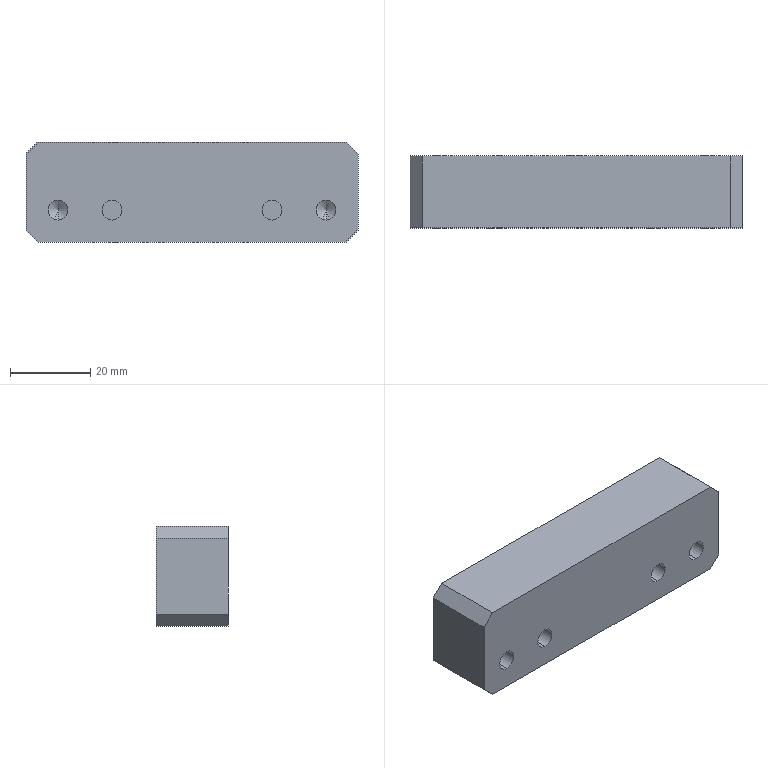Part | STEP file | PN_0043 | 1 solid | 35 faces | box 83 x 18 x 25 mm | volume 35337 mm3 | cylinder 14 | plane 13 | cone 8 | commonest cylinder face diameters 5 x14